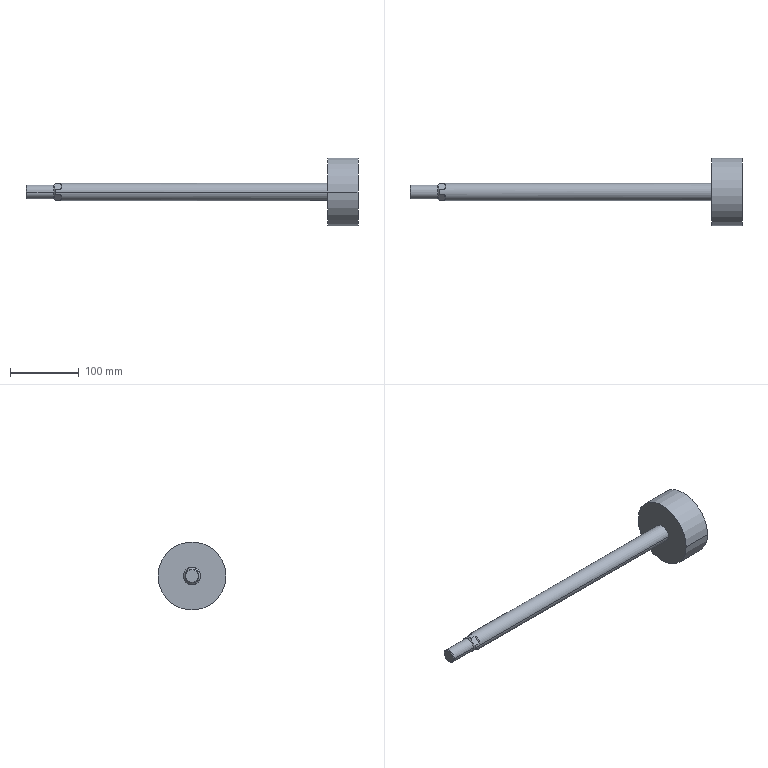Part | STEP file | _SE-100x300-CR(0)_r | 1 solid | 21 faces | box 482 x 98.6 x 98.6 mm | volume 543204 mm3 | plane 11 | cylinder 6 | cone 4 | commonest cylinder face diameters 20 x2 25 x2 98.6 x2
STEP:
#1=CARTESIAN_POINT('',(347.,-12.5,0.));
#2=VERTEX_POINT('',#1);
#3=CARTESIAN_POINT('',(347.,12.5,0.));
#4=VERTEX_POINT('',#3);
#5=CARTESIAN_POINT('',(347.,0.,0.));
#6=DIRECTION('',(-1.,0.,0.));
#7=DIRECTION('',(0.,-1.,0.));
#8=AXIS2_PLACEMENT_3D('',#5,#6,#7);
#9=CIRCLE('',#8,12.5);
#10=EDGE_CURVE('',#2,#4,#9,.T.);
#11=ORIENTED_EDGE('',*,*,#10,.T.);
#12=CARTESIAN_POINT('',(-48.5,12.5,0.));
#13=VERTEX_POINT('',#12);
#14=CARTESIAN_POINT('',(391.,12.5,0.));
#15=DIRECTION('',(-1.,0.,0.));
#16=VECTOR('',#15,1000.);
#17=LINE('',#14,#16);
#18=EDGE_CURVE('',#4,#13,#17,.T.);
#19=ORIENTED_EDGE('',*,*,#18,.T.);
#20=CARTESIAN_POINT('',(-48.5,11.976,3.58));
#21=VERTEX_POINT('',#20);
#22=CARTESIAN_POINT('',(-48.5,0.,0.));
#23=DIRECTION('',(1.,0.,0.));
#24=DIRECTION('',(0.,-1.,0.));
#25=AXIS2_PLACEMENT_3D('',#22,#23,#24);
#26=CIRCLE('',#25,12.5);
#27=EDGE_CURVE('',#13,#21,#26,.T.);
#28=ORIENTED_EDGE('',*,*,#27,.T.);
#29=CARTESIAN_POINT('',(-40.5,11.976,3.58));
#30=VERTEX_POINT('',#29);
#31=CARTESIAN_POINT('',(391.,11.976,3.58));
#32=DIRECTION('',(1.,0.,0.));
#33=VECTOR('',#32,1000.);
#34=LINE('',#31,#33);
#35=EDGE_CURVE('',#21,#30,#34,.T.);
#36=ORIENTED_EDGE('',*,*,#35,.T.);
#37=CARTESIAN_POINT('',(-40.5,3.58,11.976));
#38=VERTEX_POINT('',#37);
#39=CARTESIAN_POINT('',(-40.5,11.976,3.58));
#40=CARTESIAN_POINT('',(-38.457,10.744,7.702));
#41=CARTESIAN_POINT('',(-38.457,7.702,10.744));
#42=CARTESIAN_POINT('',(-40.5,3.58,11.976));
#43=(BOUNDED_CURVE()B_SPLINE_CURVE(3,(#39,#40,#41,#42),.UNSPECIFIED.,.F.,.F.)B_SPLINE_CURVE_WITH_KNOTS((4,4),(2.647,3.637),.UNSPECIFIED.)CURVE()GEOMETRIC_REPRESENTATION_ITEM()RATIONAL_B_SPLINE_CURVE((1.,0.92,0.92,1.))REPRESENTATION_ITEM(''));
#44=EDGE_CURVE('',#30,#38,#43,.T.);
#45=ORIENTED_EDGE('',*,*,#44,.T.);
#46=CARTESIAN_POINT('',(-48.5,3.58,11.976));
#47=VERTEX_POINT('',#46);
#48=CARTESIAN_POINT('',(391.,3.58,11.976));
#49=DIRECTION('',(-1.,0.,0.));
#50=VECTOR('',#49,1000.);
#51=LINE('',#48,#50);
#52=EDGE_CURVE('',#38,#47,#51,.T.);
#53=ORIENTED_EDGE('',*,*,#52,.T.);
#54=CARTESIAN_POINT('',(-48.5,0.,12.5));
#55=VERTEX_POINT('',#54);
#56=CARTESIAN_POINT('',(-48.5,0.,0.));
#57=DIRECTION('',(1.,0.,0.));
#58=DIRECTION('',(0.,-1.,0.));
#59=AXIS2_PLACEMENT_3D('',#56,#57,#58);
#60=CIRCLE('',#59,12.5);
#61=EDGE_CURVE('',#47,#55,#60,.T.);
#62=ORIENTED_EDGE('',*,*,#61,.T.);
#63=CARTESIAN_POINT('',(-48.5,-3.58,11.976));
#64=VERTEX_POINT('',#63);
#65=CARTESIAN_POINT('',(-48.5,0.,0.));
#66=DIRECTION('',(1.,0.,0.));
#67=DIRECTION('',(0.,-1.,0.));
#68=AXIS2_PLACEMENT_3D('',#65,#66,#67);
#69=CIRCLE('',#68,12.5);
#70=EDGE_CURVE('',#55,#64,#69,.T.);
#71=ORIENTED_EDGE('',*,*,#70,.T.);
#72=CARTESIAN_POINT('',(-40.5,-3.58,11.976));
#73=VERTEX_POINT('',#72);
#74=CARTESIAN_POINT('',(391.,-3.58,11.976));
#75=DIRECTION('',(1.,0.,0.));
#76=VECTOR('',#75,1000.);
#77=LINE('',#74,#76);
#78=EDGE_CURVE('',#64,#73,#77,.T.);
#79=ORIENTED_EDGE('',*,*,#78,.T.);
#80=CARTESIAN_POINT('',(-40.5,-11.976,3.58));
#81=VERTEX_POINT('',#80);
#82=CARTESIAN_POINT('',(-40.5,-3.58,11.976));
#83=CARTESIAN_POINT('',(-38.457,-7.702,10.744));
#84=CARTESIAN_POINT('',(-38.457,-10.744,7.702));
#85=CARTESIAN_POINT('',(-40.5,-11.976,3.58));
#86=(BOUNDED_CURVE()B_SPLINE_CURVE(3,(#82,#83,#84,#85),.UNSPECIFIED.,.F.,.F.)B_SPLINE_CURVE_WITH_KNOTS((4,4),(2.647,3.637),.UNSPECIFIED.)CURVE()GEOMETRIC_REPRESENTATION_ITEM()RATIONAL_B_SPLINE_CURVE((1.,0.92,0.92,1.))REPRESENTATION_ITEM(''));
#87=EDGE_CURVE('',#73,#81,#86,.T.);
#88=ORIENTED_EDGE('',*,*,#87,.T.);
#89=CARTESIAN_POINT('',(-48.5,-11.976,3.58));
#90=VERTEX_POINT('',#89);
#91=CARTESIAN_POINT('',(391.,-11.976,3.58));
#92=DIRECTION('',(-1.,0.,0.));
#93=VECTOR('',#92,1000.);
#94=LINE('',#91,#93);
#95=EDGE_CURVE('',#81,#90,#94,.T.);
#96=ORIENTED_EDGE('',*,*,#95,.T.);
#97=CARTESIAN_POINT('',(-48.5,-12.5,0.));
#98=VERTEX_POINT('',#97);
#99=CARTESIAN_POINT('',(-48.5,0.,0.));
#100=DIRECTION('',(1.,0.,0.));
#101=DIRECTION('',(0.,-1.,0.));
#102=AXIS2_PLACEMENT_3D('',#99,#100,#101);
#103=CIRCLE('',#102,12.5);
#104=EDGE_CURVE('',#90,#98,#103,.T.);
#105=ORIENTED_EDGE('',*,*,#104,.T.);
#106=CARTESIAN_POINT('',(391.,-12.5,0.));
#107=DIRECTION('',(-1.,0.,0.));
#108=VECTOR('',#107,1000.);
#109=LINE('',#106,#108);
#110=EDGE_CURVE('',#2,#98,#109,.T.);
#111=ORIENTED_EDGE('',*,*,#110,.F.);
#112=EDGE_LOOP('',(#11,#19,#28,#36,#45,#53,#62,#71,#79,#88,#96,#105,#111));
#113=FACE_OUTER_BOUND('',#112,.T.);
#114=CARTESIAN_POINT('',(391.,0.,0.));
#115=DIRECTION('',(-1.,0.,0.));
#116=DIRECTION('',(0.,-1.,0.));
#117=AXIS2_PLACEMENT_3D('',#114,#115,#116);
#118=CYLINDRICAL_SURFACE('',#117,12.5);
#119=ADVANCED_FACE('',(#113),#118,.T.);
#120=CARTESIAN_POINT('',(-51.,10.,0.));
#121=VERTEX_POINT('',#120);
#122=CARTESIAN_POINT('',(-51.,0.,10.));
#123=VERTEX_POINT('',#122);
#124=CARTESIAN_POINT('',(-51.,0.,0.));
#125=DIRECTION('',(1.,0.,0.));
#126=DIRECTION('',(0.,1.,0.));
#127=AXIS2_PLACEMENT_3D('',#124,#125,#126);
#128=CIRCLE('',#127,10.);
#129=EDGE_CURVE('',#121,#123,#128,.T.);
#130=ORIENTED_EDGE('',*,*,#129,.T.);
#131=CARTESIAN_POINT('',(-48.5,0.,12.5));
#132=DIRECTION('',(0.7071,0.,0.7071));
#133=VECTOR('',#132,1000.);
#134=LINE('',#131,#133);
#135=EDGE_CURVE('',#123,#55,#134,.T.);
#136=ORIENTED_EDGE('',*,*,#135,.T.);
#137=ORIENTED_EDGE('',*,*,#61,.F.);
#138=CARTESIAN_POINT('',(-48.5,3.58,11.976));
#139=CARTESIAN_POINT('',(-48.943,4.24,11.316));
#140=CARTESIAN_POINT('',(-49.316,4.914,10.642));
#141=CARTESIAN_POINT('',(-49.713,5.958,9.599));
#142=CARTESIAN_POINT('',(-49.817,6.311,9.245));
#143=CARTESIAN_POINT('',(-49.961,7.031,8.525));
#144=CARTESIAN_POINT('',(-49.999,7.401,8.156));
#145=CARTESIAN_POINT('',(-50.002,8.495,7.061));
#146=CARTESIAN_POINT('',(-49.856,9.213,6.344));
#147=CARTESIAN_POINT('',(-49.458,10.274,5.282));
#148=CARTESIAN_POINT('',(-49.296,10.624,4.933));
#149=CARTESIAN_POINT('',(-48.928,11.308,4.248));
#150=CARTESIAN_POINT('',(-48.723,11.645,3.912));
#151=CARTESIAN_POINT('',(-48.5,11.976,3.58));
#152=B_SPLINE_CURVE_WITH_KNOTS('',3,(#138,#139,#140,#141,#142,#143,#144,#145,#146,#147,#148,#149,#150,#151),.UNSPECIFIED.,.F.,.F.,(4,2,2,2,2,2,4),(0.,0.003056,0.004584,0.006112,0.009169,0.0107,0.01222),.UNSPECIFIED.);
#153=EDGE_CURVE('',#47,#21,#152,.T.);
#154=ORIENTED_EDGE('',*,*,#153,.T.);
#155=ORIENTED_EDGE('',*,*,#27,.F.);
#156=CARTESIAN_POINT('',(-48.5,11.976,-3.58));
#157=VERTEX_POINT('',#156);
#158=CARTESIAN_POINT('',(-48.5,0.,0.));
#159=DIRECTION('',(1.,0.,0.));
#160=DIRECTION('',(0.,-1.,0.));
#161=AXIS2_PLACEMENT_3D('',#158,#159,#160);
#162=CIRCLE('',#161,12.5);
#163=EDGE_CURVE('',#157,#13,#162,.T.);
#164=ORIENTED_EDGE('',*,*,#163,.F.);
#165=CARTESIAN_POINT('',(-48.5,3.58,-11.976));
#166=VERTEX_POINT('',#165);
#167=CARTESIAN_POINT('',(-48.5,11.976,-3.58));
#168=CARTESIAN_POINT('',(-48.943,11.316,-4.24));
#169=CARTESIAN_POINT('',(-49.316,10.642,-4.914));
#170=CARTESIAN_POINT('',(-49.713,9.599,-5.958));
#171=CARTESIAN_POINT('',(-49.817,9.245,-6.311));
#172=CARTESIAN_POINT('',(-49.961,8.525,-7.031));
#173=CARTESIAN_POINT('',(-49.999,8.156,-7.401));
#174=CARTESIAN_POINT('',(-50.002,7.061,-8.495));
#175=CARTESIAN_POINT('',(-49.856,6.344,-9.213));
#176=CARTESIAN_POINT('',(-49.458,5.282,-10.274));
#177=CARTESIAN_POINT('',(-49.296,4.933,-10.624));
#178=CARTESIAN_POINT('',(-48.928,4.248,-11.308));
#179=CARTESIAN_POINT('',(-48.723,3.912,-11.645));
#180=CARTESIAN_POINT('',(-48.5,3.58,-11.976));
#181=B_SPLINE_CURVE_WITH_KNOTS('',3,(#167,#168,#169,#170,#171,#172,#173,#174,#175,#176,#177,#178,#179,#180),.UNSPECIFIED.,.F.,.F.,(4,2,2,2,2,2,4),(0.,0.003056,0.004584,0.006112,0.009169,0.0107,0.01222),.UNSPECIFIED.);
#182=EDGE_CURVE('',#157,#166,#181,.T.);
#183=ORIENTED_EDGE('',*,*,#182,.T.);
#184=CARTESIAN_POINT('',(-48.5,0.,-12.5));
#185=VERTEX_POINT('',#184);
#186=CARTESIAN_POINT('',(-48.5,0.,0.));
#187=DIRECTION('',(1.,0.,0.));
#188=DIRECTION('',(0.,-1.,0.));
#189=AXIS2_PLACEMENT_3D('',#186,#187,#188);
#190=CIRCLE('',#189,12.5);
#191=EDGE_CURVE('',#185,#166,#190,.T.);
#192=ORIENTED_EDGE('',*,*,#191,.F.);
#193=CARTESIAN_POINT('',(-51.,0.,-10.));
#194=VERTEX_POINT('',#193);
#195=CARTESIAN_POINT('',(-48.5,0.,-12.5));
#196=DIRECTION('',(0.7071,0.,-0.7071));
#197=VECTOR('',#196,1000.);
#198=LINE('',#195,#197);
#199=EDGE_CURVE('',#194,#185,#198,.T.);
#200=ORIENTED_EDGE('',*,*,#199,.F.);
#201=CARTESIAN_POINT('',(-51.,0.,0.));
#202=DIRECTION('',(1.,0.,0.));
#203=DIRECTION('',(0.,1.,0.));
#204=AXIS2_PLACEMENT_3D('',#201,#202,#203);
#205=CIRCLE('',#204,10.);
#206=EDGE_CURVE('',#194,#121,#205,.T.);
#207=ORIENTED_EDGE('',*,*,#206,.T.);
#208=EDGE_LOOP('',(#130,#136,#137,#154,#155,#164,#183,#192,#200,#207));
#209=FACE_OUTER_BOUND('',#208,.T.);
#210=CARTESIAN_POINT('',(-48.5,0.,0.));
#211=DIRECTION('',(1.,0.,0.));
#212=DIRECTION('',(0.,0.,-1.));
#213=AXIS2_PLACEMENT_3D('',#210,#211,#212);
#214=CONICAL_SURFACE('',#213,12.5,0.7854);
#215=ADVANCED_FACE('',(#209),#214,.T.);
#216=ORIENTED_EDGE('',*,*,#129,.F.);
#217=CARTESIAN_POINT('',(-90.08,10.,0.));
#218=VERTEX_POINT('',#217);
#219=CARTESIAN_POINT('',(391.,10.,0.));
#220=DIRECTION('',(-1.,0.,0.));
#221=VECTOR('',#220,1000.);
#222=LINE('',#219,#221);
#223=EDGE_CURVE('',#121,#218,#222,.T.);
#224=ORIENTED_EDGE('',*,*,#223,.T.);
#225=CARTESIAN_POINT('',(-90.08,0.,10.));
#226=VERTEX_POINT('',#225);
#227=CARTESIAN_POINT('',(-90.08,0.,0.));
#228=DIRECTION('',(1.,0.,0.));
#229=DIRECTION('',(0.,-1.,0.));
#230=AXIS2_PLACEMENT_3D('',#227,#228,#229);
#231=CIRCLE('',#230,10.);
#232=EDGE_CURVE('',#218,#226,#231,.T.);
#233=ORIENTED_EDGE('',*,*,#232,.T.);
#234=CARTESIAN_POINT('',(-90.08,-10.,0.));
#235=VERTEX_POINT('',#234);
#236=CARTESIAN_POINT('',(-90.08,0.,0.));
#237=DIRECTION('',(1.,0.,0.));
#238=DIRECTION('',(0.,-1.,0.));
#239=AXIS2_PLACEMENT_3D('',#236,#237,#238);
#240=CIRCLE('',#239,10.);
#241=EDGE_CURVE('',#226,#235,#240,.T.);
#242=ORIENTED_EDGE('',*,*,#241,.T.);
#243=CARTESIAN_POINT('',(-51.,-10.,0.));
#244=VERTEX_POINT('',#243);
#245=CARTESIAN_POINT('',(391.,-10.,0.));
#246=DIRECTION('',(-1.,0.,0.));
#247=VECTOR('',#246,1000.);
#248=LINE('',#245,#247);
#249=EDGE_CURVE('',#244,#235,#248,.T.);
#250=ORIENTED_EDGE('',*,*,#249,.F.);
#251=CARTESIAN_POINT('',(-51.,0.,0.));
#252=DIRECTION('',(1.,0.,0.));
#253=DIRECTION('',(0.,1.,0.));
#254=AXIS2_PLACEMENT_3D('',#251,#252,#253);
#255=CIRCLE('',#254,10.);
#256=EDGE_CURVE('',#123,#244,#255,.T.);
#257=ORIENTED_EDGE('',*,*,#256,.F.);
#258=EDGE_LOOP('',(#216,#224,#233,#242,#250,#257));
#259=FACE_OUTER_BOUND('',#258,.T.);
#260=CARTESIAN_POINT('',(391.,0.,0.));
#261=DIRECTION('',(-1.,0.,0.));
#262=DIRECTION('',(0.,-1.,0.));
#263=AXIS2_PLACEMENT_3D('',#260,#261,#262);
#264=CYLINDRICAL_SURFACE('',#263,10.);
#265=ADVANCED_FACE('',(#259),#264,.T.);
#266=CARTESIAN_POINT('',(391.,-49.3,0.));
#267=VERTEX_POINT('',#266);
#268=CARTESIAN_POINT('',(391.,49.3,0.));
#269=VERTEX_POINT('',#268);
#270=CARTESIAN_POINT('',(391.,0.,0.));
#271=DIRECTION('',(-1.,0.,0.));
#272=DIRECTION('',(0.,-1.,0.));
#273=AXIS2_PLACEMENT_3D('',#270,#271,#272);
#274=CIRCLE('',#273,49.3);
#275=EDGE_CURVE('',#267,#269,#274,.T.);
#276=ORIENTED_EDGE('',*,*,#275,.T.);
#277=CARTESIAN_POINT('',(347.,49.3,0.));
#278=VERTEX_POINT('',#277);
#279=CARTESIAN_POINT('',(391.,49.3,0.));
#280=DIRECTION('',(-1.,0.,0.));
#281=VECTOR('',#280,1000.);
#282=LINE('',#279,#281);
#283=EDGE_CURVE('',#269,#278,#282,.T.);
#284=ORIENTED_EDGE('',*,*,#283,.T.);
#285=CARTESIAN_POINT('',(347.,-49.3,0.));
#286=VERTEX_POINT('',#285);
#287=CARTESIAN_POINT('',(347.,0.,0.));
#288=DIRECTION('',(1.,0.,0.));
#289=DIRECTION('',(0.,-1.,0.));
#290=AXIS2_PLACEMENT_3D('',#287,#288,#289);
#291=CIRCLE('',#290,49.3);
#292=EDGE_CURVE('',#278,#286,#291,.T.);
#293=ORIENTED_EDGE('',*,*,#292,.T.);
#294=CARTESIAN_POINT('',(391.,-49.3,0.));
#295=DIRECTION('',(-1.,0.,0.));
#296=VECTOR('',#295,1000.);
#297=LINE('',#294,#296);
#298=EDGE_CURVE('',#267,#286,#297,.T.);
#299=ORIENTED_EDGE('',*,*,#298,.F.);
#300=EDGE_LOOP('',(#276,#284,#293,#299));
#301=FACE_OUTER_BOUND('',#300,.T.);
#302=CARTESIAN_POINT('',(391.,0.,0.));
#303=DIRECTION('',(-1.,0.,0.));
#304=DIRECTION('',(0.,-1.,0.));
#305=AXIS2_PLACEMENT_3D('',#302,#303,#304);
#306=CYLINDRICAL_SURFACE('',#305,49.3);
#307=ADVANCED_FACE('',(#301),#306,.T.);
#308=CARTESIAN_POINT('',(-91.,0.,-9.08));
#309=VERTEX_POINT('',#308);
#310=CARTESIAN_POINT('',(-91.,0.,9.08));
#311=VERTEX_POINT('',#310);
#312=CARTESIAN_POINT('',(-91.,0.,0.));
#313=DIRECTION('',(1.,0.,0.));
#314=DIRECTION('',(0.,0.,-1.));
#315=AXIS2_PLACEMENT_3D('',#312,#313,#314);
#316=CIRCLE('',#315,9.08);
#317=EDGE_CURVE('',#309,#311,#316,.T.);
#318=ORIENTED_EDGE('',*,*,#317,.T.);
#319=CARTESIAN_POINT('',(-90.08,0.,10.));
#320=DIRECTION('',(0.7071,0.,0.7071));
#321=VECTOR('',#320,1000.);
#322=LINE('',#319,#321);
#323=EDGE_CURVE('',#311,#226,#322,.T.);
#324=ORIENTED_EDGE('',*,*,#323,.T.);
#325=ORIENTED_EDGE('',*,*,#232,.F.);
#326=CARTESIAN_POINT('',(-90.08,0.,-10.));
#327=VERTEX_POINT('',#326);
#328=CARTESIAN_POINT('',(-90.08,0.,0.));
#329=DIRECTION('',(1.,0.,0.));
#330=DIRECTION('',(0.,-1.,0.));
#331=AXIS2_PLACEMENT_3D('',#328,#329,#330);
#332=CIRCLE('',#331,10.);
#333=EDGE_CURVE('',#327,#218,#332,.T.);
#334=ORIENTED_EDGE('',*,*,#333,.F.);
#335=CARTESIAN_POINT('',(-90.08,0.,-10.));
#336=DIRECTION('',(0.7071,0.,-0.7071));
#337=VECTOR('',#336,1000.);
#338=LINE('',#335,#337);
#339=EDGE_CURVE('',#309,#327,#338,.T.);
#340=ORIENTED_EDGE('',*,*,#339,.F.);
#341=EDGE_LOOP('',(#318,#324,#325,#334,#340));
#342=FACE_OUTER_BOUND('',#341,.T.);
#343=CARTESIAN_POINT('',(-90.08,0.,0.));
#344=DIRECTION('',(1.,0.,0.));
#345=DIRECTION('',(0.,0.,-1.));
#346=AXIS2_PLACEMENT_3D('',#343,#344,#345);
#347=CONICAL_SURFACE('',#346,10.,0.7854);
#348=ADVANCED_FACE('',(#342),#347,.T.);
#349=ORIENTED_EDGE('',*,*,#18,.F.);
#350=CARTESIAN_POINT('',(347.,0.,0.));
#351=DIRECTION('',(-1.,0.,0.));
#352=DIRECTION('',(0.,-1.,0.));
#353=AXIS2_PLACEMENT_3D('',#350,#351,#352);
#354=CIRCLE('',#353,12.5);
#355=EDGE_CURVE('',#4,#2,#354,.T.);
#356=ORIENTED_EDGE('',*,*,#355,.T.);
#357=ORIENTED_EDGE('',*,*,#110,.T.);
#358=CARTESIAN_POINT('',(-48.5,-11.976,-3.58));
#359=VERTEX_POINT('',#358);
#360=CARTESIAN_POINT('',(-48.5,0.,0.));
#361=DIRECTION('',(1.,0.,0.));
#362=DIRECTION('',(0.,-1.,0.));
#363=AXIS2_PLACEMENT_3D('',#360,#361,#362);
#364=CIRCLE('',#363,12.5);
#365=EDGE_CURVE('',#98,#359,#364,.T.);
#366=ORIENTED_EDGE('',*,*,#365,.T.);
#367=CARTESIAN_POINT('',(-40.5,-11.976,-3.58));
#368=VERTEX_POINT('',#367);
#369=CARTESIAN_POINT('',(391.,-11.976,-3.58));
#370=DIRECTION('',(1.,0.,0.));
#371=VECTOR('',#370,1000.);
#372=LINE('',#369,#371);
#373=EDGE_CURVE('',#359,#368,#372,.T.);
#374=ORIENTED_EDGE('',*,*,#373,.T.);
#375=CARTESIAN_POINT('',(-40.5,-3.58,-11.976));
#376=VERTEX_POINT('',#375);
#377=CARTESIAN_POINT('',(-40.5,-11.976,-3.58));
#378=CARTESIAN_POINT('',(-38.457,-10.744,-7.702));
#379=CARTESIAN_POINT('',(-38.457,-7.702,-10.744));
#380=CARTESIAN_POINT('',(-40.5,-3.58,-11.976));
#381=(BOUNDED_CURVE()B_SPLINE_CURVE(3,(#377,#378,#379,#380),.UNSPECIFIED.,.F.,.F.)B_SPLINE_CURVE_WITH_KNOTS((4,4),(2.647,3.637),.UNSPECIFIED.)CURVE()GEOMETRIC_REPRESENTATION_ITEM()RATIONAL_B_SPLINE_CURVE((1.,0.92,0.92,1.))REPRESENTATION_ITEM(''));
#382=EDGE_CURVE('',#368,#376,#381,.T.);
#383=ORIENTED_EDGE('',*,*,#382,.T.);
#384=CARTESIAN_POINT('',(-48.5,-3.58,-11.976));
#385=VERTEX_POINT('',#384);
#386=CARTESIAN_POINT('',(391.,-3.58,-11.976));
#387=DIRECTION('',(-1.,0.,0.));
#388=VECTOR('',#387,1000.);
#389=LINE('',#386,#388);
#390=EDGE_CURVE('',#376,#385,#389,.T.);
#391=ORIENTED_EDGE('',*,*,#390,.T.);
#392=CARTESIAN_POINT('',(-48.5,0.,0.));
#393=DIRECTION('',(1.,0.,0.));
#394=DIRECTION('',(0.,-1.,0.));
#395=AXIS2_PLACEMENT_3D('',#392,#393,#394);
#396=CIRCLE('',#395,12.5);
#397=EDGE_CURVE('',#385,#185,#396,.T.);
#398=ORIENTED_EDGE('',*,*,#397,.T.);
#399=ORIENTED_EDGE('',*,*,#191,.T.);
#400=CARTESIAN_POINT('',(-40.5,3.58,-11.976));
#401=VERTEX_POINT('',#400);
#402=CARTESIAN_POINT('',(391.,3.58,-11.976));
#403=DIRECTION('',(1.,0.,0.));
#404=VECTOR('',#403,1000.);
#405=LINE('',#402,#404);
#406=EDGE_CURVE('',#166,#401,#405,.T.);
#407=ORIENTED_EDGE('',*,*,#406,.T.);
#408=CARTESIAN_POINT('',(-40.5,11.976,-3.58));
#409=VERTEX_POINT('',#408);
#410=CARTESIAN_POINT('',(-40.5,3.58,-11.976));
#411=CARTESIAN_POINT('',(-38.457,7.702,-10.744));
#412=CARTESIAN_POINT('',(-38.457,10.744,-7.702));
#413=CARTESIAN_POINT('',(-40.5,11.976,-3.58));
#414=(BOUNDED_CURVE()B_SPLINE_CURVE(3,(#410,#411,#412,#413),.UNSPECIFIED.,.F.,.F.)B_SPLINE_CURVE_WITH_KNOTS((4,4),(2.647,3.637),.UNSPECIFIED.)CURVE()GEOMETRIC_REPRESENTATION_ITEM()RATIONAL_B_SPLINE_CURVE((1.,0.92,0.92,1.))REPRESENTATION_ITEM(''));
#415=EDGE_CURVE('',#401,#409,#414,.T.);
#416=ORIENTED_EDGE('',*,*,#415,.T.);
#417=CARTESIAN_POINT('',(391.,11.976,-3.58));
#418=DIRECTION('',(-1.,0.,0.));
#419=VECTOR('',#418,1000.);
#420=LINE('',#417,#419);
#421=EDGE_CURVE('',#409,#157,#420,.T.);
#422=ORIENTED_EDGE('',*,*,#421,.T.);
#423=ORIENTED_EDGE('',*,*,#163,.T.);
#424=EDGE_LOOP('',(#349,#356,#357,#366,#374,#383,#391,#398,#399,#407,#416,#422,#423));
#425=FACE_OUTER_BOUND('',#424,.T.);
#426=CARTESIAN_POINT('',(391.,0.,0.));
#427=DIRECTION('',(-1.,0.,0.));
#428=DIRECTION('',(0.,-1.,0.));
#429=AXIS2_PLACEMENT_3D('',#426,#427,#428);
#430=CYLINDRICAL_SURFACE('',#429,12.5);
#431=ADVANCED_FACE('',(#425),#430,.T.);
#432=ORIENTED_EDGE('',*,*,#382,.F.);
#433=CARTESIAN_POINT('',(-40.5,-11.976,-3.58));
#434=DIRECTION('',(0.,0.7071,-0.7071));
#435=VECTOR('',#434,1000.);
#436=LINE('',#433,#435);
#437=EDGE_CURVE('',#368,#376,#436,.T.);
#438=ORIENTED_EDGE('',*,*,#437,.T.);
#439=EDGE_LOOP('',(#432,#438));
#440=FACE_OUTER_BOUND('',#439,.T.);
#441=CARTESIAN_POINT('',(-39.,-16.617,-1.061));
#442=DIRECTION('',(-0.7071,-0.5,-0.5));
#443=DIRECTION('',(-0.5774,0.,0.8165));
#444=AXIS2_PLACEMENT_3D('',#441,#442,#443);
#445=PLANE('',#444);
#446=ADVANCED_FACE('',(#440),#445,.T.);
#447=ORIENTED_EDGE('',*,*,#373,.F.);
#448=CARTESIAN_POINT('',(-48.5,-11.976,-3.58));
#449=CARTESIAN_POINT('',(-48.943,-11.316,-4.24));
#450=CARTESIAN_POINT('',(-49.316,-10.642,-4.914));
#451=CARTESIAN_POINT('',(-49.713,-9.599,-5.958));
#452=CARTESIAN_POINT('',(-49.817,-9.245,-6.311));
#453=CARTESIAN_POINT('',(-49.961,-8.525,-7.031));
#454=CARTESIAN_POINT('',(-49.999,-8.156,-7.401));
#455=CARTESIAN_POINT('',(-50.002,-7.061,-8.495));
#456=CARTESIAN_POINT('',(-49.856,-6.344,-9.213));
#457=CARTESIAN_POINT('',(-49.458,-5.282,-10.274));
#458=CARTESIAN_POINT('',(-49.296,-4.933,-10.624));
#459=CARTESIAN_POINT('',(-48.928,-4.248,-11.308));
#460=CARTESIAN_POINT('',(-48.723,-3.912,-11.645));
#461=CARTESIAN_POINT('',(-48.5,-3.58,-11.976));
#462=B_SPLINE_CURVE_WITH_KNOTS('',3,(#448,#449,#450,#451,#452,#453,#454,#455,#456,#457,#458,#459,#460,#461),.UNSPECIFIED.,.F.,.F.,(4,2,2,2,2,2,4),(0.,0.003056,0.004584,0.006112,0.009169,0.0107,0.01222),.UNSPECIFIED.);
#463=EDGE_CURVE('',#359,#385,#462,.T.);
#464=ORIENTED_EDGE('',*,*,#463,.T.);
#465=ORIENTED_EDGE('',*,*,#390,.F.);
#466=ORIENTED_EDGE('',*,*,#437,.F.);
#467=EDGE_LOOP('',(#447,#464,#465,#466));
#468=FACE_OUTER_BOUND('',#467,.T.);
#469=CARTESIAN_POINT('',(-40.5,-15.556,0.));
#470=DIRECTION('',(0.,-0.7071,-0.7071));
#471=DIRECTION('',(0.,0.7071,-0.7071));
#472=AXIS2_PLACEMENT_3D('',#469,#470,#471);
#473=PLANE('',#472);
#474=ADVANCED_FACE('',(#468),#473,.T.);
#475=ORIENTED_EDGE('',*,*,#135,.F.);
#476=ORIENTED_EDGE('',*,*,#256,.T.);
#477=CARTESIAN_POINT('',(-51.,0.,0.));
#478=DIRECTION('',(1.,0.,0.));
#479=DIRECTION('',(0.,1.,0.));
#480=AXIS2_PLACEMENT_3D('',#477,#478,#479);
#481=CIRCLE('',#480,10.);
#482=EDGE_CURVE('',#244,#194,#481,.T.);
#483=ORIENTED_EDGE('',*,*,#482,.T.);
#484=ORIENTED_EDGE('',*,*,#199,.T.);
#485=ORIENTED_EDGE('',*,*,#397,.F.);
#486=ORIENTED_EDGE('',*,*,#463,.F.);
#487=ORIENTED_EDGE('',*,*,#365,.F.);
#488=ORIENTED_EDGE('',*,*,#104,.F.);
#489=CARTESIAN_POINT('',(-48.5,-11.976,3.58));
#490=CARTESIAN_POINT('',(-48.943,-11.316,4.24));
#491=CARTESIAN_POINT('',(-49.316,-10.642,4.914));
#492=CARTESIAN_POINT('',(-49.713,-9.599,5.958));
#493=CARTESIAN_POINT('',(-49.817,-9.245,6.311));
#494=CARTESIAN_POINT('',(-49.961,-8.525,7.031));
#495=CARTESIAN_POINT('',(-49.999,-8.156,7.401));
#496=CARTESIAN_POINT('',(-50.002,-7.061,8.495));
#497=CARTESIAN_POINT('',(-49.856,-6.344,9.213));
#498=CARTESIAN_POINT('',(-49.458,-5.282,10.274));
#499=CARTESIAN_POINT('',(-49.296,-4.933,10.624));
#500=CARTESIAN_POINT('',(-48.928,-4.248,11.308));
#501=CARTESIAN_POINT('',(-48.723,-3.912,11.645));
#502=CARTESIAN_POINT('',(-48.5,-3.58,11.976));
#503=B_SPLINE_CURVE_WITH_KNOTS('',3,(#489,#490,#491,#492,#493,#494,#495,#496,#497,#498,#499,#500,#501,#502),.UNSPECIFIED.,.F.,.F.,(4,2,2,2,2,2,4),(0.,0.003056,0.004584,0.006112,0.009169,0.0107,0.01222),.UNSPECIFIED.);
#504=EDGE_CURVE('',#90,#64,#503,.T.);
#505=ORIENTED_EDGE('',*,*,#504,.T.);
#506=ORIENTED_EDGE('',*,*,#70,.F.);
#507=EDGE_LOOP('',(#475,#476,#483,#484,#485,#486,#487,#488,#505,#506));
#508=FACE_OUTER_BOUND('',#507,.T.);
#509=CARTESIAN_POINT('',(-48.5,0.,0.));
#510=DIRECTION('',(1.,0.,0.));
#511=DIRECTION('',(0.,0.,-1.));
#512=AXIS2_PLACEMENT_3D('',#509,#510,#511);
#513=CONICAL_SURFACE('',#512,12.5,0.7854);
#514=ADVANCED_FACE('',(#508),#513,.T.);
#515=ORIENTED_EDGE('',*,*,#78,.F.);
#516=ORIENTED_EDGE('',*,*,#504,.F.);
#517=ORIENTED_EDGE('',*,*,#95,.F.);
#518=CARTESIAN_POINT('',(-40.5,0.,15.556));
#519=DIRECTION('',(0.,0.7071,0.7071));
#520=VECTOR('',#519,1000.);
#521=LINE('',#518,#520);
#522=EDGE_CURVE('',#81,#73,#521,.T.);
#523=ORIENTED_EDGE('',*,*,#522,.T.);
#524=EDGE_LOOP('',(#515,#516,#517,#523));
#525=FACE_OUTER_BOUND('',#524,.T.);
#526=CARTESIAN_POINT('',(-40.5,0.,15.556));
#527=DIRECTION('',(0.,-0.7071,0.7071));
#528=DIRECTION('',(0.,-0.7071,-0.7071));
#529=AXIS2_PLACEMENT_3D('',#526,#527,#528);
#530=PLANE('',#529);
#531=ADVANCED_FACE('',(#525),#530,.T.);
#532=ORIENTED_EDGE('',*,*,#87,.F.);
#533=ORIENTED_EDGE('',*,*,#522,.F.);
#534=EDGE_LOOP('',(#532,#533));
#535=FACE_OUTER_BOUND('',#534,.T.);
#536=CARTESIAN_POINT('',(-39.,-1.061,16.617));
#537=DIRECTION('',(-0.7071,-0.5,0.5));
#538=DIRECTION('',(0.5774,0.,0.8165));
#539=AXIS2_PLACEMENT_3D('',#536,#537,#538);
#540=PLANE('',#539);
#541=ADVANCED_FACE('',(#535),#540,.T.);
#542=ORIENTED_EDGE('',*,*,#35,.F.);
#543=ORIENTED_EDGE('',*,*,#153,.F.);
#544=ORIENTED_EDGE('',*,*,#52,.F.);
#545=CARTESIAN_POINT('',(-40.5,0.,15.556));
#546=DIRECTION('',(0.,0.7071,-0.7071));
#547=VECTOR('',#546,1000.);
#548=LINE('',#545,#547);
#549=EDGE_CURVE('',#38,#30,#548,.T.);
#550=ORIENTED_EDGE('',*,*,#549,.T.);
#551=EDGE_LOOP('',(#542,#543,#544,#550));
#552=FACE_OUTER_BOUND('',#551,.T.);
#553=CARTESIAN_POINT('',(-94.6,0.,15.556));
#554=DIRECTION('',(0.,0.7071,0.7071));
#555=DIRECTION('',(0.,-0.7071,0.7071));
#556=AXIS2_PLACEMENT_3D('',#553,#554,#555);
#557=PLANE('',#556);
#558=ADVANCED_FACE('',(#552),#557,.T.);
#559=ORIENTED_EDGE('',*,*,#44,.F.);
#560=ORIENTED_EDGE('',*,*,#549,.F.);
#561=EDGE_LOOP('',(#559,#560));
#562=FACE_OUTER_BOUND('',#561,.T.);
#563=CARTESIAN_POINT('',(-40.5,0.,15.556));
#564=DIRECTION('',(-0.7071,0.5,0.5));
#565=DIRECTION('',(0.5774,0.,0.8165));
#566=AXIS2_PLACEMENT_3D('',#563,#564,#565);
#567=PLANE('',#566);
#568=ADVANCED_FACE('',(#562),#567,.T.);
#569=ORIENTED_EDGE('',*,*,#406,.F.);
#570=ORIENTED_EDGE('',*,*,#182,.F.);
#571=ORIENTED_EDGE('',*,*,#421,.F.);
#572=CARTESIAN_POINT('',(-40.5,15.556,0.));
#573=DIRECTION('',(0.,-0.7071,-0.7071));
#574=VECTOR('',#573,1000.);
#575=LINE('',#572,#574);
#576=EDGE_CURVE('',#409,#401,#575,.T.);
#577=ORIENTED_EDGE('',*,*,#576,.T.);
#578=EDGE_LOOP('',(#569,#570,#571,#577));
#579=FACE_OUTER_BOUND('',#578,.T.);
#580=CARTESIAN_POINT('',(-94.6,15.556,0.));
#581=DIRECTION('',(0.,0.7071,-0.7071));
#582=DIRECTION('',(0.,0.7071,0.7071));
#583=AXIS2_PLACEMENT_3D('',#580,#581,#582);
#584=PLANE('',#583);
#585=ADVANCED_FACE('',(#579),#584,.T.);
#586=ORIENTED_EDGE('',*,*,#415,.F.);
#587=ORIENTED_EDGE('',*,*,#576,.F.);
#588=EDGE_LOOP('',(#586,#587));
#589=FACE_OUTER_BOUND('',#588,.T.);
#590=CARTESIAN_POINT('',(-40.5,15.556,0.));
#591=DIRECTION('',(-0.7071,0.5,-0.5));
#592=DIRECTION('',(-0.5774,0.,0.8165));
#593=AXIS2_PLACEMENT_3D('',#590,#591,#592);
#594=PLANE('',#593);
#595=ADVANCED_FACE('',(#589),#594,.T.);
#596=ORIENTED_EDGE('',*,*,#10,.F.);
#597=ORIENTED_EDGE('',*,*,#355,.F.);
#598=EDGE_LOOP('',(#596,#597));
#599=FACE_BOUND('',#598,.T.);
#600=CARTESIAN_POINT('',(347.,0.,0.));
#601=DIRECTION('',(1.,0.,0.));
#602=DIRECTION('',(0.,-1.,0.));
#603=AXIS2_PLACEMENT_3D('',#600,#601,#602);
#604=CIRCLE('',#603,49.3);
#605=EDGE_CURVE('',#286,#278,#604,.T.);
#606=ORIENTED_EDGE('',*,*,#605,.F.);
#607=ORIENTED_EDGE('',*,*,#292,.F.);
#608=EDGE_LOOP('',(#606,#607));
#609=FACE_OUTER_BOUND('',#608,.T.);
#610=CARTESIAN_POINT('',(347.,12.5,0.));
#611=DIRECTION('',(1.,0.,0.));
#612=DIRECTION('',(0.,1.,0.));
#613=AXIS2_PLACEMENT_3D('',#610,#611,#612);
#614=PLANE('',#613);
#615=ADVANCED_FACE('',(#599,#609),#614,.F.);
#616=ORIENTED_EDGE('',*,*,#223,.F.);
#617=ORIENTED_EDGE('',*,*,#206,.F.);
#618=ORIENTED_EDGE('',*,*,#482,.F.);
#619=ORIENTED_EDGE('',*,*,#249,.T.);
#620=CARTESIAN_POINT('',(-90.08,0.,0.));
#621=DIRECTION('',(1.,0.,0.));
#622=DIRECTION('',(0.,-1.,0.));
#623=AXIS2_PLACEMENT_3D('',#620,#621,#622);
#624=CIRCLE('',#623,10.);
#625=EDGE_CURVE('',#235,#327,#624,.T.);
#626=ORIENTED_EDGE('',*,*,#625,.T.);
#627=ORIENTED_EDGE('',*,*,#333,.T.);
#628=EDGE_LOOP('',(#616,#617,#618,#619,#626,#627));
#629=FACE_OUTER_BOUND('',#628,.T.);
#630=CARTESIAN_POINT('',(391.,0.,0.));
#631=DIRECTION('',(-1.,0.,0.));
#632=DIRECTION('',(0.,-1.,0.));
#633=AXIS2_PLACEMENT_3D('',#630,#631,#632);
#634=CYLINDRICAL_SURFACE('',#633,10.);
#635=ADVANCED_FACE('',(#629),#634,.T.);
#636=ORIENTED_EDGE('',*,*,#283,.F.);
#637=CARTESIAN_POINT('',(391.,0.,0.));
#638=DIRECTION('',(-1.,0.,0.));
#639=DIRECTION('',(0.,-1.,0.));
#640=AXIS2_PLACEMENT_3D('',#637,#638,#639);
#641=CIRCLE('',#640,49.3);
#642=EDGE_CURVE('',#269,#267,#641,.T.);
#643=ORIENTED_EDGE('',*,*,#642,.T.);
#644=ORIENTED_EDGE('',*,*,#298,.T.);
#645=ORIENTED_EDGE('',*,*,#605,.T.);
#646=EDGE_LOOP('',(#636,#643,#644,#645));
#647=FACE_OUTER_BOUND('',#646,.T.);
#648=CARTESIAN_POINT('',(391.,0.,0.));
#649=DIRECTION('',(-1.,0.,0.));
#650=DIRECTION('',(0.,-1.,0.));
#651=AXIS2_PLACEMENT_3D('',#648,#649,#650);
#652=CYLINDRICAL_SURFACE('',#651,49.3);
#653=ADVANCED_FACE('',(#647),#652,.T.);
#654=ORIENTED_EDGE('',*,*,#323,.F.);
#655=CARTESIAN_POINT('',(-91.,0.,0.));
#656=DIRECTION('',(1.,0.,0.));
#657=DIRECTION('',(0.,0.,-1.));
#658=AXIS2_PLACEMENT_3D('',#655,#656,#657);
#659=CIRCLE('',#658,9.08);
#660=EDGE_CURVE('',#311,#309,#659,.T.);
#661=ORIENTED_EDGE('',*,*,#660,.T.);
#662=ORIENTED_EDGE('',*,*,#339,.T.);
#663=ORIENTED_EDGE('',*,*,#625,.F.);
#664=ORIENTED_EDGE('',*,*,#241,.F.);
#665=EDGE_LOOP('',(#654,#661,#662,#663,#664));
#666=FACE_OUTER_BOUND('',#665,.T.);
#667=CARTESIAN_POINT('',(-90.08,0.,0.));
#668=DIRECTION('',(1.,0.,0.));
#669=DIRECTION('',(0.,0.,-1.));
#670=AXIS2_PLACEMENT_3D('',#667,#668,#669);
#671=CONICAL_SURFACE('',#670,10.,0.7854);
#672=ADVANCED_FACE('',(#666),#671,.T.);
#673=ORIENTED_EDGE('',*,*,#275,.F.);
#674=ORIENTED_EDGE('',*,*,#642,.F.);
#675=EDGE_LOOP('',(#673,#674));
#676=FACE_OUTER_BOUND('',#675,.T.);
#677=CARTESIAN_POINT('',(391.,49.3,0.));
#678=DIRECTION('',(-1.,0.,0.));
#679=DIRECTION('',(0.,-1.,0.));
#680=AXIS2_PLACEMENT_3D('',#677,#678,#679);
#681=PLANE('',#680);
#682=ADVANCED_FACE('',(#676),#681,.F.);
#683=ORIENTED_EDGE('',*,*,#317,.F.);
#684=ORIENTED_EDGE('',*,*,#660,.F.);
#685=EDGE_LOOP('',(#683,#684));
#686=FACE_OUTER_BOUND('',#685,.T.);
#687=CARTESIAN_POINT('',(-91.,0.,0.));
#688=DIRECTION('',(1.,0.,0.));
#689=DIRECTION('',(0.,1.,0.));
#690=AXIS2_PLACEMENT_3D('',#687,#688,#689);
#691=PLANE('',#690);
#692=ADVANCED_FACE('',(#686),#691,.F.);
#693=CLOSED_SHELL('',(#119,#215,#265,#307,#348,#431,#446,#474,#514,#531,#541,#558,#568,#585,#595,#615,#635,#653,#672,#682,#692));
#694=MANIFOLD_SOLID_BREP('',#693);
#695=CARTESIAN_POINT('',(0.,0.,0.));
#696=DIRECTION('',(0.,0.,1.));
#697=DIRECTION('',(1.,0.,0.));
#698=AXIS2_PLACEMENT_3D('',#695,#696,#697);
#699=(LENGTH_UNIT()NAMED_UNIT(*)SI_UNIT(.MILLI.,.METRE.));
#700=UNCERTAINTY_MEASURE_WITH_UNIT(LENGTH_MEASURE(0.00001),#699,'','');
#701=(NAMED_UNIT(*)PLANE_ANGLE_UNIT()SI_UNIT($,.RADIAN.));
#702=(NAMED_UNIT(*)SI_UNIT($,.STERADIAN.)SOLID_ANGLE_UNIT());
#703=(GEOMETRIC_REPRESENTATION_CONTEXT(3)GLOBAL_UNCERTAINTY_ASSIGNED_CONTEXT((#700))GLOBAL_UNIT_ASSIGNED_CONTEXT((#699,#701,#702))REPRESENTATION_CONTEXT('',''));
#704=ADVANCED_BREP_SHAPE_REPRESENTATION('',(#694,#698),#703);